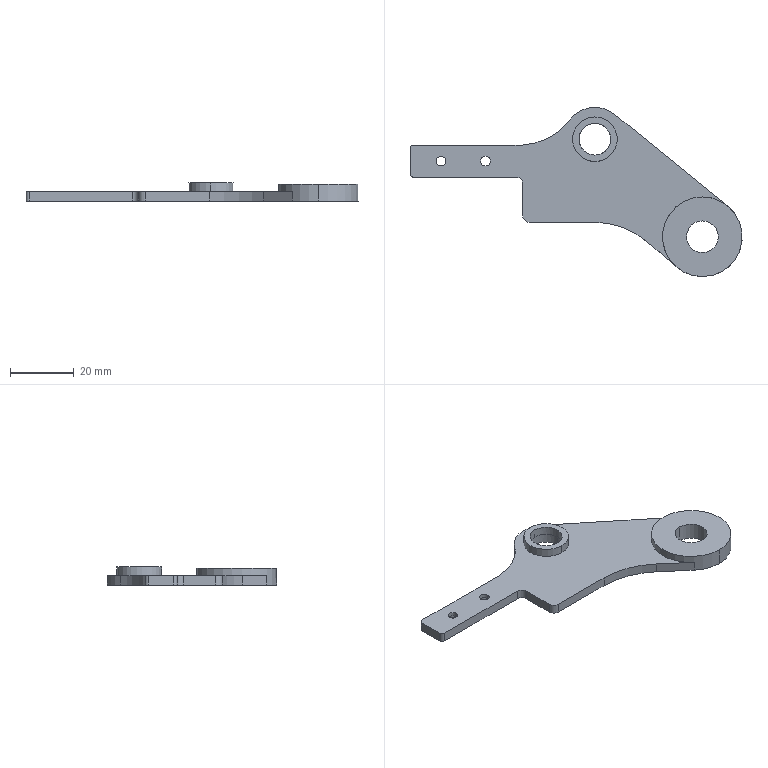Part | NX | features BREP 2, Delete Body 1, REPLACE_FACE 1 | 1 solid | 36 faces | box 104.242 x 53.12 x 5.7 mm | volume 7739 mm3 | cylinder 20 | plane 11 | cone 4 | spline 1 | commonest cylinder face diameters 10 x6 3 x4 2 x2 4 x2 14 x2 25 x2
STEP:
#1=CARTESIAN_POINT('',(-175.404,201.172,0.7));
#2=VERTEX_POINT('',#1);
#3=CARTESIAN_POINT('',(-175.404,191.172,0.7));
#4=VERTEX_POINT('',#3);
#5=CARTESIAN_POINT('',(-175.404,196.172,0.7));
#6=DIRECTION('',(0.,0.,-1.));
#7=DIRECTION('',(0.,1.,0.));
#8=AXIS2_PLACEMENT_3D('',#5,#6,#7);
#9=CIRCLE('',#8,5.);
#10=EDGE_CURVE('',#2,#4,#9,.T.);
#11=ORIENTED_EDGE('',*,*,#10,.F.);
#12=CARTESIAN_POINT('',(-175.404,201.172,-2.));
#13=VERTEX_POINT('',#12);
#14=CARTESIAN_POINT('',(-175.404,201.172,17.671));
#15=DIRECTION('',(0.,0.,-1.));
#16=VECTOR('',#15,1000.);
#17=LINE('',#14,#16);
#18=EDGE_CURVE('',#13,#2,#17,.F.);
#19=ORIENTED_EDGE('',*,*,#18,.F.);
#20=CARTESIAN_POINT('',(-170.404,196.231,-2.));
#21=VERTEX_POINT('',#20);
#22=CARTESIAN_POINT('',(-175.404,201.172,-2.));
#23=CARTESIAN_POINT('',(-174.104,201.172,-2.));
#24=CARTESIAN_POINT('',(-171.516,200.106,-2.));
#25=CARTESIAN_POINT('',(-170.419,197.53,-2.));
#26=CARTESIAN_POINT('',(-170.404,196.231,-2.));
#27=B_SPLINE_CURVE_WITH_KNOTS('',3,(#22,#23,#24,#25,#26),.UNSPECIFIED.,.F.,.F.,(4,1,4),(0.,0.5,1.),.UNSPECIFIED.);
#28=EDGE_CURVE('',#13,#21,#27,.T.);
#29=ORIENTED_EDGE('',*,*,#28,.T.);
#30=CARTESIAN_POINT('',(-174.655,191.228,-2.));
#31=VERTEX_POINT('',#30);
#32=CARTESIAN_POINT('',(-170.404,196.231,-2.));
#33=CARTESIAN_POINT('',(-170.39,195.037,-2.));
#34=CARTESIAN_POINT('',(-171.255,192.646,-2.));
#35=CARTESIAN_POINT('',(-173.475,191.407,-2.));
#36=CARTESIAN_POINT('',(-174.655,191.228,-2.));
#37=B_SPLINE_CURVE_WITH_KNOTS('',3,(#32,#33,#34,#35,#36),.UNSPECIFIED.,.F.,.F.,(4,1,4),(0.,0.5,1.),.UNSPECIFIED.);
#38=EDGE_CURVE('',#21,#31,#37,.T.);
#39=ORIENTED_EDGE('',*,*,#38,.T.);
#40=CARTESIAN_POINT('',(-175.404,191.172,-2.));
#41=VERTEX_POINT('',#40);
#42=CARTESIAN_POINT('',(-174.655,191.228,-2.));
#43=CARTESIAN_POINT('',(-174.903,191.191,-2.));
#44=CARTESIAN_POINT('',(-175.153,191.172,-2.));
#45=CARTESIAN_POINT('',(-175.404,191.172,-2.));
#46=B_SPLINE_CURVE_WITH_KNOTS('',3,(#42,#43,#44,#45),.UNSPECIFIED.,.F.,.F.,(4,4),(0.,1.),.UNSPECIFIED.);
#47=EDGE_CURVE('',#31,#41,#46,.T.);
#48=ORIENTED_EDGE('',*,*,#47,.T.);
#49=CARTESIAN_POINT('',(-175.404,191.172,17.671));
#50=DIRECTION('',(0.,0.,-1.));
#51=VECTOR('',#50,1000.);
#52=LINE('',#49,#51);
#53=EDGE_CURVE('',#41,#4,#52,.F.);
#54=ORIENTED_EDGE('',*,*,#53,.T.);
#55=EDGE_LOOP('',(#11,#19,#29,#39,#48,#54));
#56=FACE_BOUND('',#55,.T.);
#57=CARTESIAN_POINT('',(-175.404,196.172,17.671));
#58=DIRECTION('',(0.,0.,-1.));
#59=DIRECTION('',(0.,1.,0.));
#60=AXIS2_PLACEMENT_3D('',#57,#58,#59);
#61=CYLINDRICAL_SURFACE('',#60,5.);
#62=ADVANCED_FACE('',(#56),#61,.F.);
#63=CARTESIAN_POINT('',(-175.404,189.172,0.7));
#64=VERTEX_POINT('',#63);
#65=CARTESIAN_POINT('',(-175.404,203.172,0.7));
#66=VERTEX_POINT('',#65);
#67=CARTESIAN_POINT('',(-175.404,196.172,0.7));
#68=DIRECTION('',(0.,0.,-1.));
#69=DIRECTION('',(0.,1.,0.));
#70=AXIS2_PLACEMENT_3D('',#67,#68,#69);
#71=CIRCLE('',#70,7.);
#72=EDGE_CURVE('',#64,#66,#71,.T.);
#73=ORIENTED_EDGE('',*,*,#72,.T.);
#74=CARTESIAN_POINT('',(-175.404,203.172,-2.));
#75=VERTEX_POINT('',#74);
#76=CARTESIAN_POINT('',(-175.404,203.172,17.671));
#77=DIRECTION('',(0.,0.,-1.));
#78=VECTOR('',#77,1000.);
#79=LINE('',#76,#78);
#80=EDGE_CURVE('',#75,#66,#79,.F.);
#81=ORIENTED_EDGE('',*,*,#80,.F.);
#82=CARTESIAN_POINT('',(-175.404,189.172,-2.));
#83=VERTEX_POINT('',#82);
#84=CARTESIAN_POINT('',(-175.404,196.172,-2.));
#85=DIRECTION('',(0.,0.,-1.));
#86=DIRECTION('',(0.,1.,0.));
#87=AXIS2_PLACEMENT_3D('',#84,#85,#86);
#88=CIRCLE('',#87,7.);
#89=EDGE_CURVE('',#83,#75,#88,.T.);
#90=ORIENTED_EDGE('',*,*,#89,.F.);
#91=CARTESIAN_POINT('',(-175.404,189.172,17.671));
#92=DIRECTION('',(0.,0.,-1.));
#93=VECTOR('',#92,1000.);
#94=LINE('',#91,#93);
#95=EDGE_CURVE('',#83,#64,#94,.F.);
#96=ORIENTED_EDGE('',*,*,#95,.T.);
#97=EDGE_LOOP('',(#73,#81,#90,#96));
#98=FACE_BOUND('',#97,.T.);
#99=CARTESIAN_POINT('',(-175.404,196.172,17.671));
#100=DIRECTION('',(0.,0.,-1.));
#101=DIRECTION('',(0.,1.,0.));
#102=AXIS2_PLACEMENT_3D('',#99,#100,#101);
#103=CYLINDRICAL_SURFACE('',#102,7.);
#104=ADVANCED_FACE('',(#98),#103,.T.);
#105=CARTESIAN_POINT('',(-141.672,153.052,0.3));
#106=VERTEX_POINT('',#105);
#107=CARTESIAN_POINT('',(-141.672,178.052,0.3));
#108=VERTEX_POINT('',#107);
#109=CARTESIAN_POINT('',(-141.672,165.552,0.3));
#110=DIRECTION('',(0.,0.,-1.));
#111=DIRECTION('',(0.,1.,0.));
#112=AXIS2_PLACEMENT_3D('',#109,#110,#111);
#113=CIRCLE('',#112,12.5);
#114=EDGE_CURVE('',#106,#108,#113,.T.);
#115=ORIENTED_EDGE('',*,*,#114,.T.);
#116=CARTESIAN_POINT('',(-141.672,178.052,-2.));
#117=VERTEX_POINT('',#116);
#118=CARTESIAN_POINT('',(-141.672,178.052,-2.));
#119=DIRECTION('',(0.,0.,-1.));
#120=VECTOR('',#119,1000.);
#121=LINE('',#118,#120);
#122=EDGE_CURVE('',#117,#108,#121,.F.);
#123=ORIENTED_EDGE('',*,*,#122,.F.);
#124=CARTESIAN_POINT('',(-149.851,156.099,-2.));
#125=VERTEX_POINT('',#124);
#126=CARTESIAN_POINT('',(-141.672,165.552,-2.));
#127=DIRECTION('',(0.,0.,-1.));
#128=DIRECTION('',(0.,1.,0.));
#129=AXIS2_PLACEMENT_3D('',#126,#127,#128);
#130=CIRCLE('',#129,12.5);
#131=EDGE_CURVE('',#125,#117,#130,.T.);
#132=ORIENTED_EDGE('',*,*,#131,.F.);
#133=CARTESIAN_POINT('',(-149.851,156.099,-5.));
#134=VERTEX_POINT('',#133);
#135=CARTESIAN_POINT('',(-149.851,156.099,-2.));
#136=DIRECTION('',(0.,0.,-1.));
#137=VECTOR('',#136,1000.);
#138=LINE('',#135,#137);
#139=EDGE_CURVE('',#125,#134,#138,.T.);
#140=ORIENTED_EDGE('',*,*,#139,.T.);
#141=CARTESIAN_POINT('',(-141.672,153.052,-5.));
#142=VERTEX_POINT('',#141);
#143=CARTESIAN_POINT('',(-141.672,165.552,-5.));
#144=DIRECTION('',(0.,0.,-1.));
#145=DIRECTION('',(0.,1.,0.));
#146=AXIS2_PLACEMENT_3D('',#143,#144,#145);
#147=CIRCLE('',#146,12.5);
#148=EDGE_CURVE('',#142,#134,#147,.T.);
#149=ORIENTED_EDGE('',*,*,#148,.F.);
#150=CARTESIAN_POINT('',(-141.672,153.052,-2.));
#151=DIRECTION('',(0.,0.,-1.));
#152=VECTOR('',#151,1000.);
#153=LINE('',#150,#152);
#154=EDGE_CURVE('',#142,#106,#153,.F.);
#155=ORIENTED_EDGE('',*,*,#154,.T.);
#156=EDGE_LOOP('',(#115,#123,#132,#140,#149,#155));
#157=FACE_BOUND('',#156,.T.);
#158=CARTESIAN_POINT('',(-141.672,165.552,-2.));
#159=DIRECTION('',(0.,0.,-1.));
#160=DIRECTION('',(0.,1.,0.));
#161=AXIS2_PLACEMENT_3D('',#158,#159,#160);
#162=CYLINDRICAL_SURFACE('',#161,12.5);
#163=ADVANCED_FACE('',(#157),#162,.T.);
#164=CARTESIAN_POINT('',(-211.209,189.293,-2.));
#165=VERTEX_POINT('',#164);
#166=CARTESIAN_POINT('',(-208.209,189.293,-2.));
#167=VERTEX_POINT('',#166);
#168=CARTESIAN_POINT('',(-209.709,189.293,-2.));
#169=DIRECTION('',(0.,0.,-1.));
#170=DIRECTION('',(0.,1.,0.));
#171=AXIS2_PLACEMENT_3D('',#168,#169,#170);
#172=CIRCLE('',#171,1.5);
#173=EDGE_CURVE('',#165,#167,#172,.T.);
#174=ORIENTED_EDGE('',*,*,#173,.F.);
#175=CARTESIAN_POINT('',(-211.209,189.293,-3.3));
#176=VERTEX_POINT('',#175);
#177=CARTESIAN_POINT('',(-211.209,189.293,0.5));
#178=DIRECTION('',(0.,0.,-1.));
#179=VECTOR('',#178,1000.);
#180=LINE('',#177,#179);
#181=EDGE_CURVE('',#165,#176,#180,.T.);
#182=ORIENTED_EDGE('',*,*,#181,.T.);
#183=CARTESIAN_POINT('',(-208.209,189.293,-3.3));
#184=VERTEX_POINT('',#183);
#185=CARTESIAN_POINT('',(-209.709,189.293,-3.3));
#186=DIRECTION('',(0.,0.,1.));
#187=DIRECTION('',(-1.,0.,0.));
#188=AXIS2_PLACEMENT_3D('',#185,#186,#187);
#189=CIRCLE('',#188,1.5);
#190=EDGE_CURVE('',#184,#176,#189,.T.);
#191=ORIENTED_EDGE('',*,*,#190,.F.);
#192=CARTESIAN_POINT('',(-208.209,189.293,0.5));
#193=DIRECTION('',(0.,0.,-1.));
#194=VECTOR('',#193,1000.);
#195=LINE('',#192,#194);
#196=EDGE_CURVE('',#167,#184,#195,.T.);
#197=ORIENTED_EDGE('',*,*,#196,.F.);
#198=EDGE_LOOP('',(#174,#182,#191,#197));
#199=FACE_BOUND('',#198,.T.);
#200=CARTESIAN_POINT('',(-209.709,189.293,0.5));
#201=DIRECTION('',(0.,0.,-1.));
#202=DIRECTION('',(-1.,0.,0.));
#203=AXIS2_PLACEMENT_3D('',#200,#201,#202);
#204=CYLINDRICAL_SURFACE('',#203,1.5);
#205=ADVANCED_FACE('',(#199),#204,.F.);
#206=CARTESIAN_POINT('',(-225.209,189.293,-2.));
#207=VERTEX_POINT('',#206);
#208=CARTESIAN_POINT('',(-222.209,189.293,-2.));
#209=VERTEX_POINT('',#208);
#210=CARTESIAN_POINT('',(-223.709,189.293,-2.));
#211=DIRECTION('',(0.,0.,-1.));
#212=DIRECTION('',(0.,1.,0.));
#213=AXIS2_PLACEMENT_3D('',#210,#211,#212);
#214=CIRCLE('',#213,1.5);
#215=EDGE_CURVE('',#207,#209,#214,.T.);
#216=ORIENTED_EDGE('',*,*,#215,.F.);
#217=CARTESIAN_POINT('',(-225.209,189.293,-3.3));
#218=VERTEX_POINT('',#217);
#219=CARTESIAN_POINT('',(-225.209,189.293,0.5));
#220=DIRECTION('',(0.,0.,-1.));
#221=VECTOR('',#220,1000.);
#222=LINE('',#219,#221);
#223=EDGE_CURVE('',#207,#218,#222,.T.);
#224=ORIENTED_EDGE('',*,*,#223,.T.);
#225=CARTESIAN_POINT('',(-222.209,189.293,-3.3));
#226=VERTEX_POINT('',#225);
#227=CARTESIAN_POINT('',(-223.709,189.293,-3.3));
#228=DIRECTION('',(0.,0.,1.));
#229=DIRECTION('',(-1.,0.,0.));
#230=AXIS2_PLACEMENT_3D('',#227,#228,#229);
#231=CIRCLE('',#230,1.5);
#232=EDGE_CURVE('',#226,#218,#231,.T.);
#233=ORIENTED_EDGE('',*,*,#232,.F.);
#234=CARTESIAN_POINT('',(-222.209,189.293,0.5));
#235=DIRECTION('',(0.,0.,-1.));
#236=VECTOR('',#235,1000.);
#237=LINE('',#234,#236);
#238=EDGE_CURVE('',#209,#226,#237,.T.);
#239=ORIENTED_EDGE('',*,*,#238,.F.);
#240=EDGE_LOOP('',(#216,#224,#233,#239));
#241=FACE_BOUND('',#240,.T.);
#242=CARTESIAN_POINT('',(-223.709,189.293,0.5));
#243=DIRECTION('',(0.,0.,-1.));
#244=DIRECTION('',(-1.,0.,0.));
#245=AXIS2_PLACEMENT_3D('',#242,#243,#244);
#246=CYLINDRICAL_SURFACE('',#245,1.5);
#247=ADVANCED_FACE('',(#241),#246,.F.);
#248=ORIENTED_EDGE('',*,*,#190,.T.);
#249=CARTESIAN_POINT('',(-212.909,189.293,-5.));
#250=VERTEX_POINT('',#249);
#251=CARTESIAN_POINT('',(-211.209,189.293,-3.3));
#252=DIRECTION('',(-0.7071,0.,-0.7071));
#253=VECTOR('',#252,1000.);
#254=LINE('',#251,#253);
#255=EDGE_CURVE('',#176,#250,#254,.T.);
#256=ORIENTED_EDGE('',*,*,#255,.T.);
#257=CARTESIAN_POINT('',(-206.509,189.293,-5.));
#258=VERTEX_POINT('',#257);
#259=CARTESIAN_POINT('',(-209.709,189.293,-5.));
#260=DIRECTION('',(0.,0.,-1.));
#261=DIRECTION('',(0.,1.,0.));
#262=AXIS2_PLACEMENT_3D('',#259,#260,#261);
#263=CIRCLE('',#262,3.2);
#264=EDGE_CURVE('',#250,#258,#263,.T.);
#265=ORIENTED_EDGE('',*,*,#264,.T.);
#266=CARTESIAN_POINT('',(-208.209,189.293,-3.3));
#267=DIRECTION('',(0.7071,0.,-0.7071));
#268=VECTOR('',#267,1000.);
#269=LINE('',#266,#268);
#270=EDGE_CURVE('',#184,#258,#269,.T.);
#271=ORIENTED_EDGE('',*,*,#270,.F.);
#272=EDGE_LOOP('',(#248,#256,#265,#271));
#273=FACE_BOUND('',#272,.T.);
#274=CARTESIAN_POINT('',(-209.709,189.293,-3.3));
#275=DIRECTION('',(0.,0.,-1.));
#276=DIRECTION('',(-1.,0.,0.));
#277=AXIS2_PLACEMENT_3D('',#274,#275,#276);
#278=CONICAL_SURFACE('',#277,1.5,0.7854);
#279=ADVANCED_FACE('',(#273),#278,.F.);
#280=ORIENTED_EDGE('',*,*,#232,.T.);
#281=CARTESIAN_POINT('',(-226.909,189.293,-5.));
#282=VERTEX_POINT('',#281);
#283=CARTESIAN_POINT('',(-225.209,189.293,-3.3));
#284=DIRECTION('',(-0.7071,0.,-0.7071));
#285=VECTOR('',#284,1000.);
#286=LINE('',#283,#285);
#287=EDGE_CURVE('',#218,#282,#286,.T.);
#288=ORIENTED_EDGE('',*,*,#287,.T.);
#289=CARTESIAN_POINT('',(-220.509,189.293,-5.));
#290=VERTEX_POINT('',#289);
#291=CARTESIAN_POINT('',(-223.709,189.293,-5.));
#292=DIRECTION('',(0.,0.,-1.));
#293=DIRECTION('',(0.,1.,0.));
#294=AXIS2_PLACEMENT_3D('',#291,#292,#293);
#295=CIRCLE('',#294,3.2);
#296=EDGE_CURVE('',#282,#290,#295,.T.);
#297=ORIENTED_EDGE('',*,*,#296,.T.);
#298=CARTESIAN_POINT('',(-222.209,189.293,-3.3));
#299=DIRECTION('',(0.7071,0.,-0.7071));
#300=VECTOR('',#299,1000.);
#301=LINE('',#298,#300);
#302=EDGE_CURVE('',#226,#290,#301,.T.);
#303=ORIENTED_EDGE('',*,*,#302,.F.);
#304=EDGE_LOOP('',(#280,#288,#297,#303));
#305=FACE_BOUND('',#304,.T.);
#306=CARTESIAN_POINT('',(-223.709,189.293,-3.3));
#307=DIRECTION('',(0.,0.,-1.));
#308=DIRECTION('',(-1.,0.,0.));
#309=AXIS2_PLACEMENT_3D('',#306,#307,#308);
#310=CONICAL_SURFACE('',#309,1.5,0.7854);
#311=ADVANCED_FACE('',(#305),#310,.F.);
#312=CARTESIAN_POINT('',(-141.672,170.552,0.3));
#313=VERTEX_POINT('',#312);
#314=CARTESIAN_POINT('',(-141.672,160.552,0.3));
#315=VERTEX_POINT('',#314);
#316=CARTESIAN_POINT('',(-141.672,165.552,0.3));
#317=DIRECTION('',(0.,0.,-1.));
#318=DIRECTION('',(0.,1.,0.));
#319=AXIS2_PLACEMENT_3D('',#316,#317,#318);
#320=CIRCLE('',#319,5.);
#321=EDGE_CURVE('',#313,#315,#320,.T.);
#322=ORIENTED_EDGE('',*,*,#321,.F.);
#323=CARTESIAN_POINT('',(-141.672,170.552,-5.));
#324=VERTEX_POINT('',#323);
#325=CARTESIAN_POINT('',(-141.672,170.552,-2.));
#326=DIRECTION('',(0.,0.,-1.));
#327=VECTOR('',#326,1000.);
#328=LINE('',#325,#327);
#329=EDGE_CURVE('',#324,#313,#328,.F.);
#330=ORIENTED_EDGE('',*,*,#329,.F.);
#331=CARTESIAN_POINT('',(-141.672,160.552,-5.));
#332=VERTEX_POINT('',#331);
#333=CARTESIAN_POINT('',(-141.672,165.552,-5.));
#334=DIRECTION('',(0.,0.,-1.));
#335=DIRECTION('',(0.,1.,0.));
#336=AXIS2_PLACEMENT_3D('',#333,#334,#335);
#337=CIRCLE('',#336,5.);
#338=EDGE_CURVE('',#324,#332,#337,.T.);
#339=ORIENTED_EDGE('',*,*,#338,.T.);
#340=CARTESIAN_POINT('',(-141.672,160.552,-2.));
#341=DIRECTION('',(0.,0.,-1.));
#342=VECTOR('',#341,1000.);
#343=LINE('',#340,#342);
#344=EDGE_CURVE('',#332,#315,#343,.F.);
#345=ORIENTED_EDGE('',*,*,#344,.T.);
#346=EDGE_LOOP('',(#322,#330,#339,#345));
#347=FACE_BOUND('',#346,.T.);
#348=CARTESIAN_POINT('',(-141.672,165.552,-2.));
#349=DIRECTION('',(0.,0.,-1.));
#350=DIRECTION('',(0.,1.,0.));
#351=AXIS2_PLACEMENT_3D('',#348,#349,#350);
#352=CYLINDRICAL_SURFACE('',#351,5.);
#353=ADVANCED_FACE('',(#347),#352,.F.);
#354=CARTESIAN_POINT('',(-170.403,196.231,-5.));
#355=VERTEX_POINT('',#354);
#356=CARTESIAN_POINT('',(-180.403,196.114,-5.));
#357=VERTEX_POINT('',#356);
#358=CARTESIAN_POINT('',(-175.403,196.172,-5.));
#359=DIRECTION('',(0.,0.,1.));
#360=DIRECTION('',(0.,-1.,0.));
#361=AXIS2_PLACEMENT_3D('',#358,#359,#360);
#362=CIRCLE('',#361,5.);
#363=EDGE_CURVE('',#355,#357,#362,.T.);
#364=ORIENTED_EDGE('',*,*,#363,.F.);
#365=CARTESIAN_POINT('',(-170.403,196.231,-2.785));
#366=DIRECTION('',(0.,0.,1.));
#367=VECTOR('',#366,1000.);
#368=LINE('',#365,#367);
#369=EDGE_CURVE('',#21,#355,#368,.F.);
#370=ORIENTED_EDGE('',*,*,#369,.F.);
#371=ORIENTED_EDGE('',*,*,#28,.F.);
#372=CARTESIAN_POINT('',(-176.152,201.116,-2.));
#373=VERTEX_POINT('',#372);
#374=CARTESIAN_POINT('',(-175.404,201.172,-2.));
#375=CARTESIAN_POINT('',(-175.654,201.172,-2.));
#376=CARTESIAN_POINT('',(-175.904,201.153,-2.));
#377=CARTESIAN_POINT('',(-176.152,201.116,-2.));
#378=B_SPLINE_CURVE_WITH_KNOTS('',3,(#374,#375,#376,#377),.UNSPECIFIED.,.F.,.F.,(4,4),(0.,1.),.UNSPECIFIED.);
#379=EDGE_CURVE('',#373,#13,#378,.F.);
#380=ORIENTED_EDGE('',*,*,#379,.F.);
#381=CARTESIAN_POINT('',(-180.403,196.114,-2.));
#382=VERTEX_POINT('',#381);
#383=CARTESIAN_POINT('',(-176.152,201.116,-2.));
#384=CARTESIAN_POINT('',(-177.332,200.937,-2.));
#385=CARTESIAN_POINT('',(-179.552,199.698,-2.));
#386=CARTESIAN_POINT('',(-180.417,197.307,-2.));
#387=CARTESIAN_POINT('',(-180.403,196.114,-2.));
#388=B_SPLINE_CURVE_WITH_KNOTS('',3,(#383,#384,#385,#386,#387),.UNSPECIFIED.,.F.,.F.,(4,1,4),(0.,0.5,1.),.UNSPECIFIED.);
#389=EDGE_CURVE('',#382,#373,#388,.F.);
#390=ORIENTED_EDGE('',*,*,#389,.F.);
#391=CARTESIAN_POINT('',(-180.403,196.114,-2.785));
#392=DIRECTION('',(0.,0.,1.));
#393=VECTOR('',#392,1000.);
#394=LINE('',#391,#393);
#395=EDGE_CURVE('',#382,#357,#394,.F.);
#396=ORIENTED_EDGE('',*,*,#395,.T.);
#397=EDGE_LOOP('',(#364,#370,#371,#380,#390,#396));
#398=FACE_BOUND('',#397,.T.);
#399=CARTESIAN_POINT('',(-175.403,196.172,-2.785));
#400=DIRECTION('',(0.,0.,1.));
#401=DIRECTION('',(0.9999,0.01167,0.));
#402=AXIS2_PLACEMENT_3D('',#399,#400,#401);
#403=CYLINDRICAL_SURFACE('',#402,5.);
#404=ADVANCED_FACE('',(#398),#403,.F.);
#405=ORIENTED_EDGE('',*,*,#369,.T.);
#406=CARTESIAN_POINT('',(-175.403,196.172,-5.));
#407=DIRECTION('',(0.,0.,1.));
#408=DIRECTION('',(0.,-1.,0.));
#409=AXIS2_PLACEMENT_3D('',#406,#407,#408);
#410=CIRCLE('',#409,5.);
#411=EDGE_CURVE('',#357,#355,#410,.T.);
#412=ORIENTED_EDGE('',*,*,#411,.F.);
#413=ORIENTED_EDGE('',*,*,#395,.F.);
#414=CARTESIAN_POINT('',(-180.403,196.114,-2.));
#415=CARTESIAN_POINT('',(-180.388,194.815,-2.));
#416=CARTESIAN_POINT('',(-179.291,192.239,-2.));
#417=CARTESIAN_POINT('',(-176.703,191.172,-2.));
#418=CARTESIAN_POINT('',(-175.404,191.172,-2.));
#419=B_SPLINE_CURVE_WITH_KNOTS('',3,(#414,#415,#416,#417,#418),.UNSPECIFIED.,.F.,.F.,(4,1,4),(0.,0.5,1.),.UNSPECIFIED.);
#420=EDGE_CURVE('',#41,#382,#419,.F.);
#421=ORIENTED_EDGE('',*,*,#420,.F.);
#422=ORIENTED_EDGE('',*,*,#47,.F.);
#423=ORIENTED_EDGE('',*,*,#38,.F.);
#424=EDGE_LOOP('',(#405,#412,#413,#421,#422,#423));
#425=FACE_BOUND('',#424,.T.);
#426=CARTESIAN_POINT('',(-175.403,196.172,-2.785));
#427=DIRECTION('',(0.,0.,1.));
#428=DIRECTION('',(0.9999,0.01167,0.));
#429=AXIS2_PLACEMENT_3D('',#426,#427,#428);
#430=CYLINDRICAL_SURFACE('',#429,5.);
#431=ADVANCED_FACE('',(#425),#430,.F.);
#432=ORIENTED_EDGE('',*,*,#329,.T.);
#433=CARTESIAN_POINT('',(-141.672,165.552,0.3));
#434=DIRECTION('',(0.,0.,-1.));
#435=DIRECTION('',(0.,1.,0.));
#436=AXIS2_PLACEMENT_3D('',#433,#434,#435);
#437=CIRCLE('',#436,5.);
#438=EDGE_CURVE('',#315,#313,#437,.T.);
#439=ORIENTED_EDGE('',*,*,#438,.F.);
#440=ORIENTED_EDGE('',*,*,#344,.F.);
#441=CARTESIAN_POINT('',(-141.672,165.552,-5.));
#442=DIRECTION('',(0.,0.,-1.));
#443=DIRECTION('',(0.,1.,0.));
#444=AXIS2_PLACEMENT_3D('',#441,#442,#443);
#445=CIRCLE('',#444,5.);
#446=EDGE_CURVE('',#332,#324,#445,.T.);
#447=ORIENTED_EDGE('',*,*,#446,.T.);
#448=EDGE_LOOP('',(#432,#439,#440,#447));
#449=FACE_BOUND('',#448,.T.);
#450=CARTESIAN_POINT('',(-141.672,165.552,-2.));
#451=DIRECTION('',(0.,0.,-1.));
#452=DIRECTION('',(0.,1.,0.));
#453=AXIS2_PLACEMENT_3D('',#450,#451,#452);
#454=CYLINDRICAL_SURFACE('',#453,5.);
#455=ADVANCED_FACE('',(#449),#454,.F.);
#456=ORIENTED_EDGE('',*,*,#287,.F.);
#457=CARTESIAN_POINT('',(-223.709,189.293,-3.3));
#458=DIRECTION('',(0.,0.,1.));
#459=DIRECTION('',(-1.,0.,0.));
#460=AXIS2_PLACEMENT_3D('',#457,#458,#459);
#461=CIRCLE('',#460,1.5);
#462=EDGE_CURVE('',#218,#226,#461,.T.);
#463=ORIENTED_EDGE('',*,*,#462,.T.);
#464=ORIENTED_EDGE('',*,*,#302,.T.);
#465=CARTESIAN_POINT('',(-223.709,189.293,-5.));
#466=DIRECTION('',(0.,0.,-1.));
#467=DIRECTION('',(0.,1.,0.));
#468=AXIS2_PLACEMENT_3D('',#465,#466,#467);
#469=CIRCLE('',#468,3.2);
#470=EDGE_CURVE('',#290,#282,#469,.T.);
#471=ORIENTED_EDGE('',*,*,#470,.T.);
#472=EDGE_LOOP('',(#456,#463,#464,#471));
#473=FACE_BOUND('',#472,.T.);
#474=CARTESIAN_POINT('',(-223.709,189.293,-3.3));
#475=DIRECTION('',(0.,0.,-1.));
#476=DIRECTION('',(-1.,0.,0.));
#477=AXIS2_PLACEMENT_3D('',#474,#475,#476);
#478=CONICAL_SURFACE('',#477,1.5,0.7854);
#479=ADVANCED_FACE('',(#473),#478,.F.);
#480=ORIENTED_EDGE('',*,*,#255,.F.);
#481=CARTESIAN_POINT('',(-209.709,189.293,-3.3));
#482=DIRECTION('',(0.,0.,1.));
#483=DIRECTION('',(-1.,0.,0.));
#484=AXIS2_PLACEMENT_3D('',#481,#482,#483);
#485=CIRCLE('',#484,1.5);
#486=EDGE_CURVE('',#176,#184,#485,.T.);
#487=ORIENTED_EDGE('',*,*,#486,.T.);
#488=ORIENTED_EDGE('',*,*,#270,.T.);
#489=CARTESIAN_POINT('',(-209.709,189.293,-5.));
#490=DIRECTION('',(0.,0.,-1.));
#491=DIRECTION('',(0.,1.,0.));
#492=AXIS2_PLACEMENT_3D('',#489,#490,#491);
#493=CIRCLE('',#492,3.2);
#494=EDGE_CURVE('',#258,#250,#493,.T.);
#495=ORIENTED_EDGE('',*,*,#494,.T.);
#496=EDGE_LOOP('',(#480,#487,#488,#495));
#497=FACE_BOUND('',#496,.T.);
#498=CARTESIAN_POINT('',(-209.709,189.293,-3.3));
#499=DIRECTION('',(0.,0.,-1.));
#500=DIRECTION('',(-1.,0.,0.));
#501=AXIS2_PLACEMENT_3D('',#498,#499,#500);
#502=CONICAL_SURFACE('',#501,1.5,0.7854);
#503=ADVANCED_FACE('',(#497),#502,.F.);
#504=ORIENTED_EDGE('',*,*,#114,.F.);
#505=CARTESIAN_POINT('',(-141.672,165.552,0.3));
#506=DIRECTION('',(0.,0.,-1.));
#507=DIRECTION('',(0.,1.,0.));
#508=AXIS2_PLACEMENT_3D('',#505,#506,#507);
#509=CIRCLE('',#508,12.5);
#510=EDGE_CURVE('',#108,#106,#509,.T.);
#511=ORIENTED_EDGE('',*,*,#510,.F.);
#512=EDGE_LOOP('',(#504,#511));
#513=FACE_BOUND('',#512,.T.);
#514=ORIENTED_EDGE('',*,*,#438,.T.);
#515=ORIENTED_EDGE('',*,*,#321,.T.);
#516=EDGE_LOOP('',(#514,#515));
#517=FACE_BOUND('',#516,.T.);
#518=CARTESIAN_POINT('',(-146.593,163.872,0.3));
#519=DIRECTION('',(0.,0.,1.));
#520=DIRECTION('',(-1.,0.,0.));
#521=AXIS2_PLACEMENT_3D('',#518,#519,#520);
#522=PLANE('',#521);
#523=ADVANCED_FACE('',(#513,#517),#522,.T.);
#524=ORIENTED_EDGE('',*,*,#411,.T.);
#525=ORIENTED_EDGE('',*,*,#363,.T.);
#526=EDGE_LOOP('',(#524,#525));
#527=FACE_BOUND('',#526,.T.);
#528=CARTESIAN_POINT('',(-133.791,175.255,-5.));
#529=VERTEX_POINT('',#528);
#530=CARTESIAN_POINT('',(-169.098,203.934,-5.));
#531=VERTEX_POINT('',#530);
#532=CARTESIAN_POINT('',(32.582,40.112,-5.));
#533=DIRECTION('',(-0.7762,0.6305,0.));
#534=VECTOR('',#533,1000.);
#535=LINE('',#532,#534);
#536=EDGE_CURVE('',#529,#531,#535,.T.);
#537=ORIENTED_EDGE('',*,*,#536,.F.);
#538=CARTESIAN_POINT('',(-141.672,165.552,-5.));
#539=DIRECTION('',(0.,0.,-1.));
#540=DIRECTION('',(0.,1.,0.));
#541=AXIS2_PLACEMENT_3D('',#538,#539,#540);
#542=CIRCLE('',#541,12.5);
#543=EDGE_CURVE('',#529,#142,#542,.T.);
#544=ORIENTED_EDGE('',*,*,#543,.T.);
#545=ORIENTED_EDGE('',*,*,#148,.T.);
#546=CARTESIAN_POINT('',(-158.769,163.815,-5.));
#547=VERTEX_POINT('',#546);
#548=CARTESIAN_POINT('',(-149.851,156.099,-5.));
#549=DIRECTION('',(-0.7563,0.6543,0.));
#550=VECTOR('',#549,1000.);
#551=LINE('',#548,#550);
#552=EDGE_CURVE('',#134,#547,#551,.T.);
#553=ORIENTED_EDGE('',*,*,#552,.T.);
#554=CARTESIAN_POINT('',(-175.761,170.145,-5.));
#555=VERTEX_POINT('',#554);
#556=CARTESIAN_POINT('',(-175.761,144.174,-5.));
#557=DIRECTION('',(0.,0.,-1.));
#558=DIRECTION('',(1.,0.,0.));
#559=AXIS2_PLACEMENT_3D('',#556,#557,#558);
#560=CIRCLE('',#559,25.971);
#561=EDGE_CURVE('',#555,#547,#560,.T.);
#562=ORIENTED_EDGE('',*,*,#561,.F.);
#563=CARTESIAN_POINT('',(-196.068,170.145,-5.));
#564=VERTEX_POINT('',#563);
#565=CARTESIAN_POINT('',(-175.761,170.145,-5.));
#566=DIRECTION('',(1.,0.,0.));
#567=VECTOR('',#566,1000.);
#568=LINE('',#565,#567);
#569=EDGE_CURVE('',#564,#555,#568,.T.);
#570=ORIENTED_EDGE('',*,*,#569,.F.);
#571=CARTESIAN_POINT('',(-198.068,172.145,-5.));
#572=VERTEX_POINT('',#571);
#573=CARTESIAN_POINT('',(-196.068,172.145,-5.));
#574=DIRECTION('',(0.,0.,1.));
#575=DIRECTION('',(0.,1.,0.));
#576=AXIS2_PLACEMENT_3D('',#573,#574,#575);
#577=CIRCLE('',#576,2.);
#578=EDGE_CURVE('',#572,#564,#577,.T.);
#579=ORIENTED_EDGE('',*,*,#578,.F.);
#580=CARTESIAN_POINT('',(-198.068,182.293,-5.));
#581=VERTEX_POINT('',#580);
#582=CARTESIAN_POINT('',(-198.068,170.145,-5.));
#583=DIRECTION('',(0.,-1.,0.));
#584=VECTOR('',#583,1000.);
#585=LINE('',#582,#584);
#586=EDGE_CURVE('',#581,#572,#585,.T.);
#587=ORIENTED_EDGE('',*,*,#586,.F.);
#588=CARTESIAN_POINT('',(-200.068,184.293,-5.));
#589=VERTEX_POINT('',#588);
#590=CARTESIAN_POINT('',(-200.068,182.293,-5.));
#591=DIRECTION('',(0.,0.,-1.));
#592=DIRECTION('',(0.,1.,0.));
#593=AXIS2_PLACEMENT_3D('',#590,#591,#592);
#594=CIRCLE('',#593,2.);
#595=EDGE_CURVE('',#589,#581,#594,.T.);
#596=ORIENTED_EDGE('',*,*,#595,.F.);
#597=CARTESIAN_POINT('',(-232.414,184.293,-5.));
#598=VERTEX_POINT('',#597);
#599=CARTESIAN_POINT('',(-141.672,184.293,-5.));
#600=DIRECTION('',(1.,0.,0.));
#601=VECTOR('',#600,1000.);
#602=LINE('',#599,#601);
#603=EDGE_CURVE('',#598,#589,#602,.T.);
#604=ORIENTED_EDGE('',*,*,#603,.F.);
#605=CARTESIAN_POINT('',(-233.414,185.293,-5.));
#606=VERTEX_POINT('',#605);
#607=CARTESIAN_POINT('',(-232.414,185.293,-5.));
#608=DIRECTION('',(0.,0.,1.));
#609=DIRECTION('',(0.,1.,0.));
#610=AXIS2_PLACEMENT_3D('',#607,#608,#609);
#611=CIRCLE('',#610,1.);
#612=EDGE_CURVE('',#606,#598,#611,.T.);
#613=ORIENTED_EDGE('',*,*,#612,.F.);
#614=CARTESIAN_POINT('',(-233.414,193.293,-5.));
#615=VERTEX_POINT('',#614);
#616=CARTESIAN_POINT('',(-233.414,185.793,-5.));
#617=DIRECTION('',(0.,-1.,0.));
#618=VECTOR('',#617,1000.);
#619=LINE('',#616,#618);
#620=EDGE_CURVE('',#615,#606,#619,.T.);
#621=ORIENTED_EDGE('',*,*,#620,.F.);
#622=CARTESIAN_POINT('',(-232.414,194.293,-5.));
#623=VERTEX_POINT('',#622);
#624=CARTESIAN_POINT('',(-232.414,193.293,-5.));
#625=DIRECTION('',(0.,0.,1.));
#626=DIRECTION('',(0.,1.,0.));
#627=AXIS2_PLACEMENT_3D('',#624,#625,#626);
#628=CIRCLE('',#627,1.);
#629=EDGE_CURVE('',#623,#615,#628,.T.);
#630=ORIENTED_EDGE('',*,*,#629,.F.);
#631=CARTESIAN_POINT('',(-198.567,194.293,-5.));
#632=VERTEX_POINT('',#631);
#633=CARTESIAN_POINT('',(-214.519,194.293,-5.));
#634=DIRECTION('',(1.,0.,0.));
#635=VECTOR('',#634,1000.);
#636=LINE('',#633,#635);
#637=EDGE_CURVE('',#623,#632,#636,.T.);
#638=ORIENTED_EDGE('',*,*,#637,.T.);
#639=CARTESIAN_POINT('',(-183.399,202.177,-5.));
#640=VERTEX_POINT('',#639);
#641=CARTESIAN_POINT('',(-198.567,194.293,-5.));
#642=CARTESIAN_POINT('',(-188.816,194.965,-5.));
#643=CARTESIAN_POINT('',(-183.399,202.177,-5.));
#644=B_SPLINE_CURVE_WITH_KNOTS('',2,(#641,#642,#643),.UNSPECIFIED.,.F.,.F.,(3,3),(0.,1.),.PIECEWISE_BEZIER_KNOTS.);
#645=EDGE_CURVE('',#632,#640,#644,.T.);
#646=ORIENTED_EDGE('',*,*,#645,.T.);
#647=CARTESIAN_POINT('',(-175.403,196.172,-5.));
#648=DIRECTION('',(0.,0.,1.));
#649=DIRECTION('',(1.,0.,0.));
#650=AXIS2_PLACEMENT_3D('',#647,#648,#649);
#651=CIRCLE('',#650,10.);
#652=EDGE_CURVE('',#531,#640,#651,.T.);
#653=ORIENTED_EDGE('',*,*,#652,.F.);
#654=EDGE_LOOP('',(#537,#544,#545,#553,#562,#570,#579,#587,#596,#604,#613,#621,#630,#638,#646,#653));
#655=FACE_BOUND('',#654,.T.);
#656=ORIENTED_EDGE('',*,*,#446,.F.);
#657=ORIENTED_EDGE('',*,*,#338,.F.);
#658=EDGE_LOOP('',(#656,#657));
#659=FACE_BOUND('',#658,.T.);
#660=ORIENTED_EDGE('',*,*,#494,.F.);
#661=ORIENTED_EDGE('',*,*,#264,.F.);
#662=EDGE_LOOP('',(#660,#661));
#663=FACE_BOUND('',#662,.T.);
#664=ORIENTED_EDGE('',*,*,#470,.F.);
#665=ORIENTED_EDGE('',*,*,#296,.F.);
#666=EDGE_LOOP('',(#664,#665));
#667=FACE_BOUND('',#666,.T.);
#668=CARTESIAN_POINT('',(-141.672,165.552,-5.));
#669=DIRECTION('',(0.,0.,1.));
#670=DIRECTION('',(-1.,0.,0.));
#671=AXIS2_PLACEMENT_3D('',#668,#669,#670);
#672=PLANE('',#671);
#673=ADVANCED_FACE('',(#527,#655,#659,#663,#667),#672,.F.);
#674=ORIENTED_EDGE('',*,*,#223,.F.);
#675=CARTESIAN_POINT('',(-223.709,189.293,-2.));
#676=DIRECTION('',(0.,0.,-1.));
#677=DIRECTION('',(0.,1.,0.));
#678=AXIS2_PLACEMENT_3D('',#675,#676,#677);
#679=CIRCLE('',#678,1.5);
#680=EDGE_CURVE('',#209,#207,#679,.T.);
#681=ORIENTED_EDGE('',*,*,#680,.F.);
#682=ORIENTED_EDGE('',*,*,#238,.T.);
#683=ORIENTED_EDGE('',*,*,#462,.F.);
#684=EDGE_LOOP('',(#674,#681,#682,#683));
#685=FACE_BOUND('',#684,.T.);
#686=CARTESIAN_POINT('',(-223.709,189.293,0.5));
#687=DIRECTION('',(0.,0.,-1.));
#688=DIRECTION('',(-1.,0.,0.));
#689=AXIS2_PLACEMENT_3D('',#686,#687,#688);
#690=CYLINDRICAL_SURFACE('',#689,1.5);
#691=ADVANCED_FACE('',(#685),#690,.F.);
#692=ORIENTED_EDGE('',*,*,#181,.F.);
#693=CARTESIAN_POINT('',(-209.709,189.293,-2.));
#694=DIRECTION('',(0.,0.,-1.));
#695=DIRECTION('',(0.,1.,0.));
#696=AXIS2_PLACEMENT_3D('',#693,#694,#695);
#697=CIRCLE('',#696,1.5);
#698=EDGE_CURVE('',#167,#165,#697,.T.);
#699=ORIENTED_EDGE('',*,*,#698,.F.);
#700=ORIENTED_EDGE('',*,*,#196,.T.);
#701=ORIENTED_EDGE('',*,*,#486,.F.);
#702=EDGE_LOOP('',(#692,#699,#700,#701));
#703=FACE_BOUND('',#702,.T.);
#704=CARTESIAN_POINT('',(-209.709,189.293,0.5));
#705=DIRECTION('',(0.,0.,-1.));
#706=DIRECTION('',(-1.,0.,0.));
#707=AXIS2_PLACEMENT_3D('',#704,#705,#706);
#708=CYLINDRICAL_SURFACE('',#707,1.5);
#709=ADVANCED_FACE('',(#703),#708,.F.);
#710=CARTESIAN_POINT('',(-232.414,194.293,-2.));
#711=VERTEX_POINT('',#710);
#712=CARTESIAN_POINT('',(-198.567,194.293,-2.));
#713=VERTEX_POINT('',#712);
#714=CARTESIAN_POINT('',(-214.519,194.293,-2.));
#715=DIRECTION('',(1.,0.,0.));
#716=VECTOR('',#715,1000.);
#717=LINE('',#714,#716);
#718=EDGE_CURVE('',#711,#713,#717,.T.);
#719=ORIENTED_EDGE('',*,*,#718,.T.);
#720=CARTESIAN_POINT('',(-198.567,194.293,-2.));
#721=DIRECTION('',(0.,0.,1.));
#722=VECTOR('',#721,1000.);
#723=LINE('',#720,#722);
#724=EDGE_CURVE('',#632,#713,#723,.T.);
#725=ORIENTED_EDGE('',*,*,#724,.F.);
#726=ORIENTED_EDGE('',*,*,#637,.F.);
#727=CARTESIAN_POINT('',(-232.414,194.293,-5.));
#728=DIRECTION('',(0.,0.,-1.));
#729=VECTOR('',#728,1000.);
#730=LINE('',#727,#729);
#731=EDGE_CURVE('',#711,#623,#730,.T.);
#732=ORIENTED_EDGE('',*,*,#731,.F.);
#733=EDGE_LOOP('',(#719,#725,#726,#732));
#734=FACE_BOUND('',#733,.T.);
#735=CARTESIAN_POINT('',(-214.519,194.293,-2.));
#736=DIRECTION('',(0.,-1.,0.));
#737=DIRECTION('',(0.,0.,1.));
#738=AXIS2_PLACEMENT_3D('',#735,#736,#737);
#739=PLANE('',#738);
#740=ADVANCED_FACE('',(#734),#739,.F.);
#741=CARTESIAN_POINT('',(-233.414,193.293,-2.));
#742=VERTEX_POINT('',#741);
#743=CARTESIAN_POINT('',(-232.414,193.293,-2.));
#744=DIRECTION('',(0.,0.,-1.));
#745=DIRECTION('',(0.,1.,0.));
#746=AXIS2_PLACEMENT_3D('',#743,#744,#745);
#747=CIRCLE('',#746,1.);
#748=EDGE_CURVE('',#742,#711,#747,.T.);
#749=ORIENTED_EDGE('',*,*,#748,.T.);
#750=ORIENTED_EDGE('',*,*,#731,.T.);
#751=ORIENTED_EDGE('',*,*,#629,.T.);
#752=CARTESIAN_POINT('',(-233.414,193.293,-2.));
#753=DIRECTION('',(0.,0.,1.));
#754=VECTOR('',#753,1000.);
#755=LINE('',#752,#754);
#756=EDGE_CURVE('',#615,#742,#755,.T.);
#757=ORIENTED_EDGE('',*,*,#756,.T.);
#758=EDGE_LOOP('',(#749,#750,#751,#757));
#759=FACE_BOUND('',#758,.T.);
#760=CARTESIAN_POINT('',(-232.414,193.293,-2.));
#761=DIRECTION('',(0.,0.,1.));
#762=DIRECTION('',(0.,-1.,0.));
#763=AXIS2_PLACEMENT_3D('',#760,#761,#762);
#764=CYLINDRICAL_SURFACE('',#763,1.);
#765=ADVANCED_FACE('',(#759),#764,.T.);
#766=CARTESIAN_POINT('',(-233.414,185.293,-2.));
#767=VERTEX_POINT('',#766);
#768=CARTESIAN_POINT('',(-233.414,185.793,-2.));
#769=DIRECTION('',(0.,-1.,0.));
#770=VECTOR('',#769,1000.);
#771=LINE('',#768,#770);
#772=EDGE_CURVE('',#742,#767,#771,.T.);
#773=ORIENTED_EDGE('',*,*,#772,.F.);
#774=ORIENTED_EDGE('',*,*,#756,.F.);
#775=ORIENTED_EDGE('',*,*,#620,.T.);
#776=CARTESIAN_POINT('',(-233.414,185.293,-5.));
#777=DIRECTION('',(0.,0.,-1.));
#778=VECTOR('',#777,1000.);
#779=LINE('',#776,#778);
#780=EDGE_CURVE('',#767,#606,#779,.T.);
#781=ORIENTED_EDGE('',*,*,#780,.F.);
#782=EDGE_LOOP('',(#773,#774,#775,#781));
#783=FACE_BOUND('',#782,.T.);
#784=CARTESIAN_POINT('',(-233.414,185.793,-2.));
#785=DIRECTION('',(-1.,0.,0.));
#786=DIRECTION('',(0.,0.,-1.));
#787=AXIS2_PLACEMENT_3D('',#784,#785,#786);
#788=PLANE('',#787);
#789=ADVANCED_FACE('',(#783),#788,.T.);
#790=CARTESIAN_POINT('',(-232.414,184.293,-2.));
#791=VERTEX_POINT('',#790);
#792=CARTESIAN_POINT('',(-232.414,185.293,-2.));
#793=DIRECTION('',(0.,0.,-1.));
#794=DIRECTION('',(0.,1.,0.));
#795=AXIS2_PLACEMENT_3D('',#792,#793,#794);
#796=CIRCLE('',#795,1.);
#797=EDGE_CURVE('',#791,#767,#796,.T.);
#798=ORIENTED_EDGE('',*,*,#797,.T.);
#799=ORIENTED_EDGE('',*,*,#780,.T.);
#800=ORIENTED_EDGE('',*,*,#612,.T.);
#801=CARTESIAN_POINT('',(-232.414,184.293,-2.));
#802=DIRECTION('',(0.,0.,1.));
#803=VECTOR('',#802,1000.);
#804=LINE('',#801,#803);
#805=EDGE_CURVE('',#598,#791,#804,.T.);
#806=ORIENTED_EDGE('',*,*,#805,.T.);
#807=EDGE_LOOP('',(#798,#799,#800,#806));
#808=FACE_BOUND('',#807,.T.);
#809=CARTESIAN_POINT('',(-232.414,185.293,-2.));
#810=DIRECTION('',(0.,0.,1.));
#811=DIRECTION('',(0.,-1.,0.));
#812=AXIS2_PLACEMENT_3D('',#809,#810,#811);
#813=CYLINDRICAL_SURFACE('',#812,1.);
#814=ADVANCED_FACE('',(#808),#813,.T.);
#815=CARTESIAN_POINT('',(-200.068,184.293,-2.));
#816=VERTEX_POINT('',#815);
#817=CARTESIAN_POINT('',(-141.672,184.293,-2.));
#818=DIRECTION('',(1.,0.,0.));
#819=VECTOR('',#818,1000.);
#820=LINE('',#817,#819);
#821=EDGE_CURVE('',#791,#816,#820,.T.);
#822=ORIENTED_EDGE('',*,*,#821,.F.);
#823=ORIENTED_EDGE('',*,*,#805,.F.);
#824=ORIENTED_EDGE('',*,*,#603,.T.);
#825=CARTESIAN_POINT('',(-200.068,184.293,-5.));
#826=DIRECTION('',(0.,0.,-1.));
#827=VECTOR('',#826,1000.);
#828=LINE('',#825,#827);
#829=EDGE_CURVE('',#816,#589,#828,.T.);
#830=ORIENTED_EDGE('',*,*,#829,.F.);
#831=EDGE_LOOP('',(#822,#823,#824,#830));
#832=FACE_BOUND('',#831,.T.);
#833=CARTESIAN_POINT('',(-233.936,184.293,-5.));
#834=DIRECTION('',(0.,1.,0.));
#835=DIRECTION('',(-1.,0.,0.));
#836=AXIS2_PLACEMENT_3D('',#833,#834,#835);
#837=PLANE('',#836);
#838=ADVANCED_FACE('',(#832),#837,.F.);
#839=CARTESIAN_POINT('',(-198.068,182.293,-2.));
#840=VERTEX_POINT('',#839);
#841=CARTESIAN_POINT('',(-200.068,182.293,-2.));
#842=DIRECTION('',(0.,0.,1.));
#843=DIRECTION('',(0.,1.,0.));
#844=AXIS2_PLACEMENT_3D('',#841,#842,#843);
#845=CIRCLE('',#844,2.);
#846=EDGE_CURVE('',#840,#816,#845,.T.);
#847=ORIENTED_EDGE('',*,*,#846,.T.);
#848=ORIENTED_EDGE('',*,*,#829,.T.);
#849=ORIENTED_EDGE('',*,*,#595,.T.);
#850=CARTESIAN_POINT('',(-198.068,182.293,42.968));
#851=DIRECTION('',(0.,0.,1.));
#852=VECTOR('',#851,1000.);
#853=LINE('',#850,#852);
#854=EDGE_CURVE('',#581,#840,#853,.T.);
#855=ORIENTED_EDGE('',*,*,#854,.T.);
#856=EDGE_LOOP('',(#847,#848,#849,#855));
#857=FACE_BOUND('',#856,.T.);
#858=CARTESIAN_POINT('',(-200.068,182.293,-5.));
#859=DIRECTION('',(0.,0.,-1.));
#860=DIRECTION('',(0.,1.,0.));
#861=AXIS2_PLACEMENT_3D('',#858,#859,#860);
#862=CYLINDRICAL_SURFACE('',#861,2.);
#863=ADVANCED_FACE('',(#857),#862,.F.);
#864=CARTESIAN_POINT('',(-198.068,172.145,-2.));
#865=VERTEX_POINT('',#864);
#866=CARTESIAN_POINT('',(-198.068,170.145,-2.));
#867=DIRECTION('',(0.,-1.,0.));
#868=VECTOR('',#867,1000.);
#869=LINE('',#866,#868);
#870=EDGE_CURVE('',#840,#865,#869,.T.);
#871=ORIENTED_EDGE('',*,*,#870,.F.);
#872=ORIENTED_EDGE('',*,*,#854,.F.);
#873=ORIENTED_EDGE('',*,*,#586,.T.);
#874=CARTESIAN_POINT('',(-198.068,172.145,42.968));
#875=DIRECTION('',(0.,0.,-1.));
#876=VECTOR('',#875,1000.);
#877=LINE('',#874,#876);
#878=EDGE_CURVE('',#865,#572,#877,.T.);
#879=ORIENTED_EDGE('',*,*,#878,.F.);
#880=EDGE_LOOP('',(#871,#872,#873,#879));
#881=FACE_BOUND('',#880,.T.);
#882=CARTESIAN_POINT('',(-198.068,170.145,42.968));
#883=DIRECTION('',(-1.,0.,0.));
#884=DIRECTION('',(0.,0.,-1.));
#885=AXIS2_PLACEMENT_3D('',#882,#883,#884);
#886=PLANE('',#885);
#887=ADVANCED_FACE('',(#881),#886,.T.);
#888=CARTESIAN_POINT('',(-196.068,170.145,-2.));
#889=VERTEX_POINT('',#888);
#890=CARTESIAN_POINT('',(-196.068,172.145,-2.));
#891=DIRECTION('',(0.,0.,-1.));
#892=DIRECTION('',(0.,1.,0.));
#893=AXIS2_PLACEMENT_3D('',#890,#891,#892);
#894=CIRCLE('',#893,2.);
#895=EDGE_CURVE('',#889,#865,#894,.T.);
#896=ORIENTED_EDGE('',*,*,#895,.T.);
#897=ORIENTED_EDGE('',*,*,#878,.T.);
#898=ORIENTED_EDGE('',*,*,#578,.T.);
#899=CARTESIAN_POINT('',(-196.068,170.145,42.968));
#900=DIRECTION('',(0.,0.,1.));
#901=VECTOR('',#900,1000.);
#902=LINE('',#899,#901);
#903=EDGE_CURVE('',#564,#889,#902,.T.);
#904=ORIENTED_EDGE('',*,*,#903,.T.);
#905=EDGE_LOOP('',(#896,#897,#898,#904));
#906=FACE_BOUND('',#905,.T.);
#907=CARTESIAN_POINT('',(-196.068,172.145,42.968));
#908=DIRECTION('',(0.,0.,-1.));
#909=DIRECTION('',(-1.,0.,0.));
#910=AXIS2_PLACEMENT_3D('',#907,#908,#909);
#911=CYLINDRICAL_SURFACE('',#910,2.);
#912=ADVANCED_FACE('',(#906),#911,.T.);
#913=ORIENTED_EDGE('',*,*,#569,.T.);
#914=CARTESIAN_POINT('',(-175.761,170.145,-2.));
#915=VERTEX_POINT('',#914);
#916=CARTESIAN_POINT('',(-175.761,170.145,42.968));
#917=DIRECTION('',(0.,0.,-1.));
#918=VECTOR('',#917,1000.);
#919=LINE('',#916,#918);
#920=EDGE_CURVE('',#915,#555,#919,.T.);
#921=ORIENTED_EDGE('',*,*,#920,.F.);
#922=CARTESIAN_POINT('',(-175.761,170.145,-2.));
#923=DIRECTION('',(1.,0.,0.));
#924=VECTOR('',#923,1000.);
#925=LINE('',#922,#924);
#926=EDGE_CURVE('',#889,#915,#925,.T.);
#927=ORIENTED_EDGE('',*,*,#926,.F.);
#928=ORIENTED_EDGE('',*,*,#903,.F.);
#929=EDGE_LOOP('',(#913,#921,#927,#928));
#930=FACE_BOUND('',#929,.T.);
#931=CARTESIAN_POINT('',(-175.761,170.145,42.968));
#932=DIRECTION('',(0.,-1.,0.));
#933=DIRECTION('',(1.,0.,0.));
#934=AXIS2_PLACEMENT_3D('',#931,#932,#933);
#935=PLANE('',#934);
#936=ADVANCED_FACE('',(#930),#935,.T.);
#937=ORIENTED_EDGE('',*,*,#920,.T.);
#938=ORIENTED_EDGE('',*,*,#561,.T.);
#939=CARTESIAN_POINT('',(-158.769,163.815,-2.));
#940=VERTEX_POINT('',#939);
#941=CARTESIAN_POINT('',(-158.769,163.815,42.968));
#942=DIRECTION('',(0.,0.,-1.));
#943=VECTOR('',#942,1000.);
#944=LINE('',#941,#943);
#945=EDGE_CURVE('',#940,#547,#944,.T.);
#946=ORIENTED_EDGE('',*,*,#945,.F.);
#947=CARTESIAN_POINT('',(-175.761,144.174,-2.));
#948=DIRECTION('',(0.,0.,-1.));
#949=DIRECTION('',(0.,1.,0.));
#950=AXIS2_PLACEMENT_3D('',#947,#948,#949);
#951=CIRCLE('',#950,25.971);
#952=EDGE_CURVE('',#915,#940,#951,.T.);
#953=ORIENTED_EDGE('',*,*,#952,.F.);
#954=EDGE_LOOP('',(#937,#938,#946,#953));
#955=FACE_BOUND('',#954,.T.);
#956=CARTESIAN_POINT('',(-175.761,144.174,42.968));
#957=DIRECTION('',(0.,0.,-1.));
#958=DIRECTION('',(-1.,0.,0.));
#959=AXIS2_PLACEMENT_3D('',#956,#957,#958);
#960=CYLINDRICAL_SURFACE('',#959,25.971);
#961=ADVANCED_FACE('',(#955),#960,.F.);
#962=ORIENTED_EDGE('',*,*,#552,.F.);
#963=ORIENTED_EDGE('',*,*,#139,.F.);
#964=CARTESIAN_POINT('',(-149.851,156.099,-2.));
#965=DIRECTION('',(-0.7563,0.6543,0.));
#966=VECTOR('',#965,1000.);
#967=LINE('',#964,#966);
#968=EDGE_CURVE('',#125,#940,#967,.T.);
#969=ORIENTED_EDGE('',*,*,#968,.T.);
#970=ORIENTED_EDGE('',*,*,#945,.T.);
#971=EDGE_LOOP('',(#962,#963,#969,#970));
#972=FACE_BOUND('',#971,.T.);
#973=CARTESIAN_POINT('',(-149.851,156.099,-2.));
#974=DIRECTION('',(0.6543,0.7563,0.));
#975=DIRECTION('',(0.,0.,1.));
#976=AXIS2_PLACEMENT_3D('',#973,#974,#975);
#977=PLANE('',#976);
#978=ADVANCED_FACE('',(#972),#977,.F.);
#979=ORIENTED_EDGE('',*,*,#122,.T.);
#980=ORIENTED_EDGE('',*,*,#510,.T.);
#981=ORIENTED_EDGE('',*,*,#154,.F.);
#982=ORIENTED_EDGE('',*,*,#543,.F.);
#983=CARTESIAN_POINT('',(-133.791,175.255,-2.));
#984=VERTEX_POINT('',#983);
#985=CARTESIAN_POINT('',(-133.791,175.255,-2.));
#986=DIRECTION('',(0.,0.,-1.));
#987=VECTOR('',#986,1000.);
#988=LINE('',#985,#987);
#989=EDGE_CURVE('',#984,#529,#988,.T.);
#990=ORIENTED_EDGE('',*,*,#989,.F.);
#991=CARTESIAN_POINT('',(-141.672,165.552,-2.));
#992=DIRECTION('',(0.,0.,-1.));
#993=DIRECTION('',(0.,1.,0.));
#994=AXIS2_PLACEMENT_3D('',#991,#992,#993);
#995=CIRCLE('',#994,12.5);
#996=EDGE_CURVE('',#117,#984,#995,.T.);
#997=ORIENTED_EDGE('',*,*,#996,.F.);
#998=EDGE_LOOP('',(#979,#980,#981,#982,#990,#997));
#999=FACE_BOUND('',#998,.T.);
#1000=CARTESIAN_POINT('',(-141.672,165.552,-2.));
#1001=DIRECTION('',(0.,0.,-1.));
#1002=DIRECTION('',(0.,1.,0.));
#1003=AXIS2_PLACEMENT_3D('',#1000,#1001,#1002);
#1004=CYLINDRICAL_SURFACE('',#1003,12.5);
#1005=ADVANCED_FACE('',(#999),#1004,.T.);
#1006=ORIENTED_EDGE('',*,*,#536,.T.);
#1007=CARTESIAN_POINT('',(-169.098,203.934,-2.));
#1008=VERTEX_POINT('',#1007);
#1009=CARTESIAN_POINT('',(-169.098,203.934,-2.));
#1010=DIRECTION('',(0.,0.,-1.));
#1011=VECTOR('',#1010,1000.);
#1012=LINE('',#1009,#1011);
#1013=EDGE_CURVE('',#1008,#531,#1012,.T.);
#1014=ORIENTED_EDGE('',*,*,#1013,.F.);
#1015=CARTESIAN_POINT('',(32.582,40.112,-2.));
#1016=DIRECTION('',(-0.7762,0.6305,0.));
#1017=VECTOR('',#1016,1000.);
#1018=LINE('',#1015,#1017);
#1019=EDGE_CURVE('',#984,#1008,#1018,.T.);
#1020=ORIENTED_EDGE('',*,*,#1019,.F.);
#1021=ORIENTED_EDGE('',*,*,#989,.T.);
#1022=EDGE_LOOP('',(#1006,#1014,#1020,#1021));
#1023=FACE_BOUND('',#1022,.T.);
#1024=CARTESIAN_POINT('',(32.582,40.112,-2.));
#1025=DIRECTION('',(0.6305,0.7762,0.));
#1026=DIRECTION('',(0.,0.,1.));
#1027=AXIS2_PLACEMENT_3D('',#1024,#1025,#1026);
#1028=PLANE('',#1027);
#1029=ADVANCED_FACE('',(#1023),#1028,.T.);
#1030=ORIENTED_EDGE('',*,*,#652,.T.);
#1031=CARTESIAN_POINT('',(-183.399,202.177,-2.));
#1032=VERTEX_POINT('',#1031);
#1033=CARTESIAN_POINT('',(-183.399,202.177,-2.));
#1034=DIRECTION('',(0.,0.,-1.));
#1035=VECTOR('',#1034,1000.);
#1036=LINE('',#1033,#1035);
#1037=EDGE_CURVE('',#1032,#640,#1036,.T.);
#1038=ORIENTED_EDGE('',*,*,#1037,.F.);
#1039=CARTESIAN_POINT('',(-175.403,196.172,-2.));
#1040=DIRECTION('',(0.,0.,1.));
#1041=DIRECTION('',(0.,1.,0.));
#1042=AXIS2_PLACEMENT_3D('',#1039,#1040,#1041);
#1043=CIRCLE('',#1042,10.);
#1044=EDGE_CURVE('',#1008,#1032,#1043,.T.);
#1045=ORIENTED_EDGE('',*,*,#1044,.F.);
#1046=ORIENTED_EDGE('',*,*,#1013,.T.);
#1047=EDGE_LOOP('',(#1030,#1038,#1045,#1046));
#1048=FACE_BOUND('',#1047,.T.);
#1049=CARTESIAN_POINT('',(-175.403,196.172,26.284));
#1050=DIRECTION('',(0.,0.,-1.));
#1051=DIRECTION('',(-1.,0.,0.));
#1052=AXIS2_PLACEMENT_3D('',#1049,#1050,#1051);
#1053=CYLINDRICAL_SURFACE('',#1052,10.);
#1054=ADVANCED_FACE('',(#1048),#1053,.T.);
#1055=CARTESIAN_POINT('',(-198.567,194.293,-2.));
#1056=CARTESIAN_POINT('',(-188.816,194.965,-2.));
#1057=CARTESIAN_POINT('',(-183.399,202.177,-2.));
#1058=B_SPLINE_CURVE_WITH_KNOTS('',2,(#1055,#1056,#1057),.UNSPECIFIED.,.F.,.F.,(3,3),(0.,1.),.PIECEWISE_BEZIER_KNOTS.);
#1059=EDGE_CURVE('',#713,#1032,#1058,.T.);
#1060=ORIENTED_EDGE('',*,*,#1059,.T.);
#1061=ORIENTED_EDGE('',*,*,#1037,.T.);
#1062=ORIENTED_EDGE('',*,*,#645,.F.);
#1063=ORIENTED_EDGE('',*,*,#724,.T.);
#1064=EDGE_LOOP('',(#1060,#1061,#1062,#1063));
#1065=FACE_BOUND('',#1064,.T.);
#1066=CARTESIAN_POINT('',(-183.399,202.177,-2.));
#1067=CARTESIAN_POINT('',(-183.399,202.177,-5.));
#1068=CARTESIAN_POINT('',(-188.816,194.965,-2.));
#1069=CARTESIAN_POINT('',(-188.816,194.965,-5.));
#1070=CARTESIAN_POINT('',(-198.567,194.293,-2.));
#1071=CARTESIAN_POINT('',(-198.567,194.293,-5.));
#1072=B_SPLINE_SURFACE_WITH_KNOTS('',2,1,((#1066,#1067),(#1068,#1069),(#1070,#1071)),.SURF_OF_LINEAR_EXTRUSION.,.F.,.F.,.F.,(3,3),(2,2),(0.,1.),(0.,1.),.PIECEWISE_BEZIER_KNOTS.);
#1073=ADVANCED_FACE('',(#1065),#1072,.F.);
#1074=ORIENTED_EDGE('',*,*,#1059,.F.);
#1075=ORIENTED_EDGE('',*,*,#718,.F.);
#1076=ORIENTED_EDGE('',*,*,#748,.F.);
#1077=ORIENTED_EDGE('',*,*,#772,.T.);
#1078=ORIENTED_EDGE('',*,*,#797,.F.);
#1079=ORIENTED_EDGE('',*,*,#821,.T.);
#1080=ORIENTED_EDGE('',*,*,#846,.F.);
#1081=ORIENTED_EDGE('',*,*,#870,.T.);
#1082=ORIENTED_EDGE('',*,*,#895,.F.);
#1083=ORIENTED_EDGE('',*,*,#926,.T.);
#1084=ORIENTED_EDGE('',*,*,#952,.T.);
#1085=ORIENTED_EDGE('',*,*,#968,.F.);
#1086=ORIENTED_EDGE('',*,*,#131,.T.);
#1087=ORIENTED_EDGE('',*,*,#996,.T.);
#1088=ORIENTED_EDGE('',*,*,#1019,.T.);
#1089=ORIENTED_EDGE('',*,*,#1044,.T.);
#1090=EDGE_LOOP('',(#1074,#1075,#1076,#1077,#1078,#1079,#1080,#1081,#1082,#1083,#1084,#1085,#1086,#1087,#1088,#1089));
#1091=FACE_BOUND('',#1090,.T.);
#1092=ORIENTED_EDGE('',*,*,#89,.T.);
#1093=CARTESIAN_POINT('',(-175.404,196.172,-2.));
#1094=DIRECTION('',(0.,0.,-1.));
#1095=DIRECTION('',(0.,1.,0.));
#1096=AXIS2_PLACEMENT_3D('',#1093,#1094,#1095);
#1097=CIRCLE('',#1096,7.);
#1098=EDGE_CURVE('',#75,#83,#1097,.T.);
#1099=ORIENTED_EDGE('',*,*,#1098,.T.);
#1100=EDGE_LOOP('',(#1092,#1099));
#1101=FACE_BOUND('',#1100,.T.);
#1102=ORIENTED_EDGE('',*,*,#698,.T.);
#1103=ORIENTED_EDGE('',*,*,#173,.T.);
#1104=EDGE_LOOP('',(#1102,#1103));
#1105=FACE_BOUND('',#1104,.T.);
#1106=ORIENTED_EDGE('',*,*,#680,.T.);
#1107=ORIENTED_EDGE('',*,*,#215,.T.);
#1108=EDGE_LOOP('',(#1106,#1107));
#1109=FACE_BOUND('',#1108,.T.);
#1110=CARTESIAN_POINT('',(-141.672,165.552,-2.));
#1111=DIRECTION('',(0.,0.,1.));
#1112=DIRECTION('',(-1.,0.,0.));
#1113=AXIS2_PLACEMENT_3D('',#1110,#1111,#1112);
#1114=PLANE('',#1113);
#1115=ADVANCED_FACE('',(#1091,#1101,#1105,#1109),#1114,.T.);
#1116=ORIENTED_EDGE('',*,*,#80,.T.);
#1117=CARTESIAN_POINT('',(-175.404,196.172,0.7));
#1118=DIRECTION('',(0.,0.,-1.));
#1119=DIRECTION('',(0.,1.,0.));
#1120=AXIS2_PLACEMENT_3D('',#1117,#1118,#1119);
#1121=CIRCLE('',#1120,7.);
#1122=EDGE_CURVE('',#66,#64,#1121,.T.);
#1123=ORIENTED_EDGE('',*,*,#1122,.T.);
#1124=ORIENTED_EDGE('',*,*,#95,.F.);
#1125=ORIENTED_EDGE('',*,*,#1098,.F.);
#1126=EDGE_LOOP('',(#1116,#1123,#1124,#1125));
#1127=FACE_BOUND('',#1126,.T.);
#1128=CARTESIAN_POINT('',(-175.404,196.172,17.671));
#1129=DIRECTION('',(0.,0.,-1.));
#1130=DIRECTION('',(0.,1.,0.));
#1131=AXIS2_PLACEMENT_3D('',#1128,#1129,#1130);
#1132=CYLINDRICAL_SURFACE('',#1131,7.);
#1133=ADVANCED_FACE('',(#1127),#1132,.T.);
#1134=ORIENTED_EDGE('',*,*,#18,.T.);
#1135=CARTESIAN_POINT('',(-175.404,196.172,0.7));
#1136=DIRECTION('',(0.,0.,-1.));
#1137=DIRECTION('',(0.,1.,0.));
#1138=AXIS2_PLACEMENT_3D('',#1135,#1136,#1137);
#1139=CIRCLE('',#1138,5.);
#1140=EDGE_CURVE('',#4,#2,#1139,.T.);
#1141=ORIENTED_EDGE('',*,*,#1140,.F.);
#1142=ORIENTED_EDGE('',*,*,#53,.F.);
#1143=ORIENTED_EDGE('',*,*,#420,.T.);
#1144=ORIENTED_EDGE('',*,*,#389,.T.);
#1145=ORIENTED_EDGE('',*,*,#379,.T.);
#1146=EDGE_LOOP('',(#1134,#1141,#1142,#1143,#1144,#1145));
#1147=FACE_BOUND('',#1146,.T.);
#1148=CARTESIAN_POINT('',(-175.404,196.172,17.671));
#1149=DIRECTION('',(0.,0.,-1.));
#1150=DIRECTION('',(0.,1.,0.));
#1151=AXIS2_PLACEMENT_3D('',#1148,#1149,#1150);
#1152=CYLINDRICAL_SURFACE('',#1151,5.);
#1153=ADVANCED_FACE('',(#1147),#1152,.F.);
#1154=ORIENTED_EDGE('',*,*,#72,.F.);
#1155=ORIENTED_EDGE('',*,*,#1122,.F.);
#1156=EDGE_LOOP('',(#1154,#1155));
#1157=FACE_BOUND('',#1156,.T.);
#1158=ORIENTED_EDGE('',*,*,#1140,.T.);
#1159=ORIENTED_EDGE('',*,*,#10,.T.);
#1160=EDGE_LOOP('',(#1158,#1159));
#1161=FACE_BOUND('',#1160,.T.);
#1162=CARTESIAN_POINT('',(-171.015,198.961,0.7));
#1163=DIRECTION('',(0.,0.,1.));
#1164=DIRECTION('',(-1.,0.,0.));
#1165=AXIS2_PLACEMENT_3D('',#1162,#1163,#1164);
#1166=PLANE('',#1165);
#1167=ADVANCED_FACE('',(#1157,#1161),#1166,.T.);
#1168=CLOSED_SHELL('',(#62,#104,#163,#205,#247,#279,#311,#353,#404,#431,#455,#479,#503,#523,#673,#691,#709,#740,#765,#789,#814,#838,#863,#887,#912,#936,#961,#978,#1005,#1029,#1054,#1073,#1115,#1133,#1153,#1167));
#1169=MANIFOLD_SOLID_BREP('',#1168);
#1170=(LENGTH_UNIT()NAMED_UNIT(*)SI_UNIT(.MILLI.,.METRE.));
#1171=UNCERTAINTY_MEASURE_WITH_UNIT(LENGTH_MEASURE(0.0508),#1170,'','');
#1172=(NAMED_UNIT(*)PLANE_ANGLE_UNIT()SI_UNIT($,.RADIAN.));
#1173=(NAMED_UNIT(*)SI_UNIT($,.STERADIAN.)SOLID_ANGLE_UNIT());
#1174=(GEOMETRIC_REPRESENTATION_CONTEXT(3)GLOBAL_UNCERTAINTY_ASSIGNED_CONTEXT((#1171))GLOBAL_UNIT_ASSIGNED_CONTEXT((#1170,#1172,#1173))REPRESENTATION_CONTEXT('',''));
#1175=ADVANCED_BREP_SHAPE_REPRESENTATION('',(#1169),#1174);